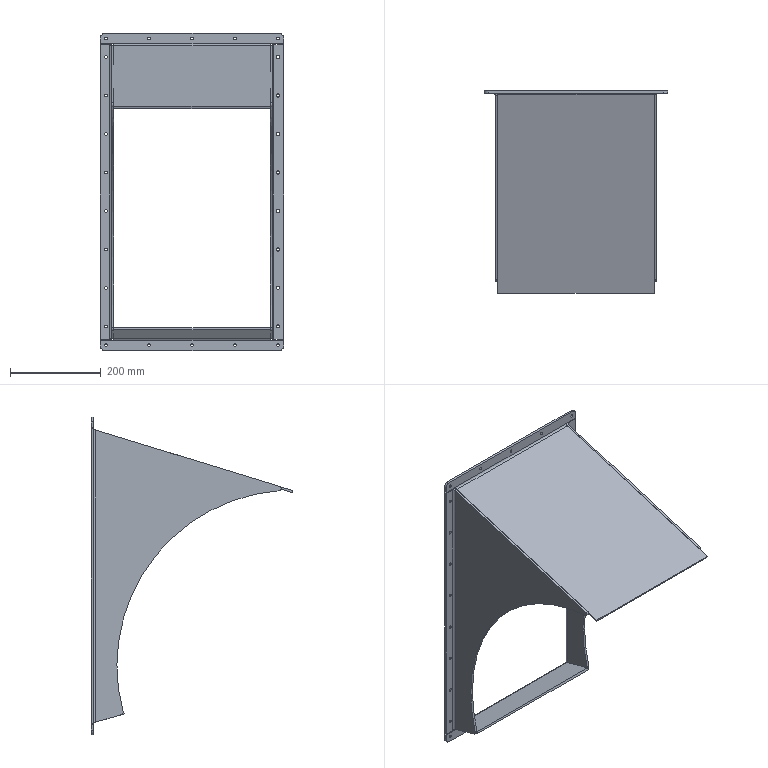Part | SolidWorks | 4 solids | 172 faces | box 405 x 446.049 x 700.825 mm | volume 2089258 mm3 | cylinder 70 | cone 52 | plane 46 | spline 4 | commonest cylinder face diameters 6 x37 7 x16 10 x7 20 x7 775 x2 16 x1